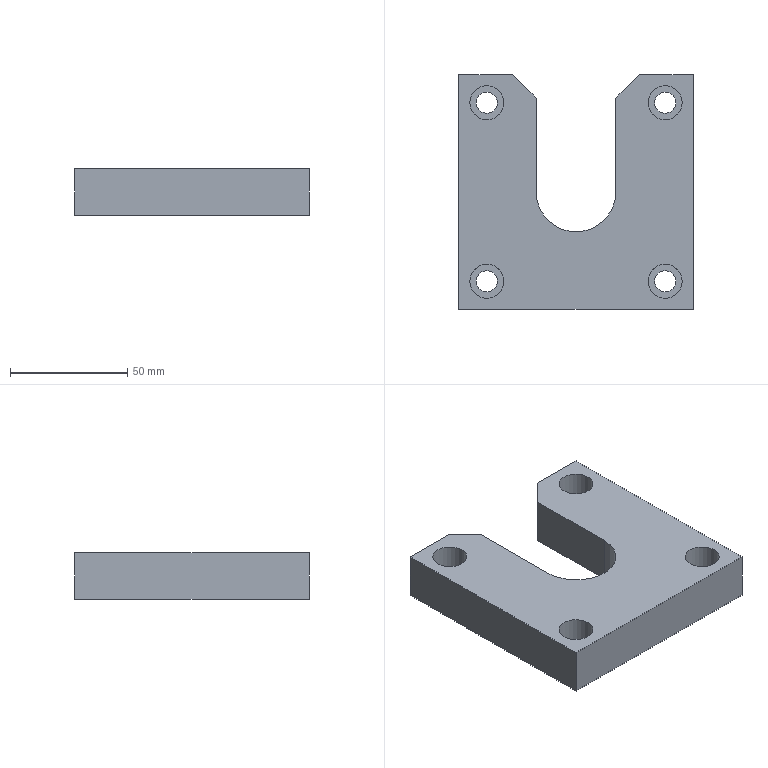Part | STEP file | lll_id890_x_t | 1 solid | 24 faces | box 100 x 100 x 20 mm | volume 145352 mm3 | plane 15 | cylinder 9 | commonest cylinder face diameters 9.009 x4 14.508 x4 34 x1
STEP:
#1=CARTESIAN_POINT('',(3772.181,632.,-360.));
#2=VERTEX_POINT('',#1);
#3=CARTESIAN_POINT('',(3779.435,632.,-360.));
#4=DIRECTION('',(0.,0.,1.));
#5=DIRECTION('',(-1.,0.,0.));
#6=AXIS2_PLACEMENT_3D('',#3,#4,#5);
#7=CIRCLE('',#6,7.254);
#8=EDGE_CURVE('',#2,#2,#7,.T.);
#9=ORIENTED_EDGE('',*,*,#8,.F.);
#10=EDGE_LOOP('',(#9));
#11=FACE_BOUND('',#10,.T.);
#12=CARTESIAN_POINT('',(3848.181,708.,-360.));
#13=VERTEX_POINT('',#12);
#14=CARTESIAN_POINT('',(3855.435,708.,-360.));
#15=DIRECTION('',(0.,0.,1.));
#16=DIRECTION('',(-1.,0.,0.));
#17=AXIS2_PLACEMENT_3D('',#14,#15,#16);
#18=CIRCLE('',#17,7.254);
#19=EDGE_CURVE('',#13,#13,#18,.T.);
#20=ORIENTED_EDGE('',*,*,#19,.F.);
#21=EDGE_LOOP('',(#20));
#22=FACE_BOUND('',#21,.T.);
#23=CARTESIAN_POINT('',(3790.435,720.,-360.));
#24=VERTEX_POINT('',#23);
#25=CARTESIAN_POINT('',(3767.435,720.,-360.));
#26=VERTEX_POINT('',#25);
#27=CARTESIAN_POINT('',(3817.435,720.,-360.));
#28=DIRECTION('',(-1.,0.,0.));
#29=VECTOR('',#28,1.);
#30=LINE('',#27,#29);
#31=EDGE_CURVE('',#24,#26,#30,.T.);
#32=ORIENTED_EDGE('',*,*,#31,.T.);
#33=CARTESIAN_POINT('',(3767.435,620.,-360.));
#34=VERTEX_POINT('',#33);
#35=CARTESIAN_POINT('',(3767.435,662.5,-360.));
#36=DIRECTION('',(0.,-1.,0.));
#37=VECTOR('',#36,1.);
#38=LINE('',#35,#37);
#39=EDGE_CURVE('',#26,#34,#38,.T.);
#40=ORIENTED_EDGE('',*,*,#39,.T.);
#41=CARTESIAN_POINT('',(3867.435,620.,-360.));
#42=VERTEX_POINT('',#41);
#43=CARTESIAN_POINT('',(3817.435,620.,-360.));
#44=DIRECTION('',(1.,0.,0.));
#45=VECTOR('',#44,1.);
#46=LINE('',#43,#45);
#47=EDGE_CURVE('',#34,#42,#46,.T.);
#48=ORIENTED_EDGE('',*,*,#47,.T.);
#49=CARTESIAN_POINT('',(3867.435,720.,-360.));
#50=VERTEX_POINT('',#49);
#51=CARTESIAN_POINT('',(3867.435,662.5,-360.));
#52=DIRECTION('',(0.,1.,0.));
#53=VECTOR('',#52,1.);
#54=LINE('',#51,#53);
#55=EDGE_CURVE('',#42,#50,#54,.T.);
#56=ORIENTED_EDGE('',*,*,#55,.T.);
#57=CARTESIAN_POINT('',(3844.435,720.,-360.));
#58=VERTEX_POINT('',#57);
#59=CARTESIAN_POINT('',(3817.435,720.,-360.));
#60=DIRECTION('',(-1.,0.,0.));
#61=VECTOR('',#60,1.);
#62=LINE('',#59,#61);
#63=EDGE_CURVE('',#50,#58,#62,.T.);
#64=ORIENTED_EDGE('',*,*,#63,.T.);
#65=CARTESIAN_POINT('',(3834.435,710.,-360.));
#66=VERTEX_POINT('',#65);
#67=CARTESIAN_POINT('',(3802.185,677.75,-360.));
#68=DIRECTION('',(-0.7071,-0.7071,0.));
#69=VECTOR('',#68,1.);
#70=LINE('',#67,#69);
#71=EDGE_CURVE('',#58,#66,#70,.T.);
#72=ORIENTED_EDGE('',*,*,#71,.T.);
#73=CARTESIAN_POINT('',(3834.435,670.,-360.));
#74=VERTEX_POINT('',#73);
#75=CARTESIAN_POINT('',(3834.435,662.5,-360.));
#76=DIRECTION('',(0.,1.,0.));
#77=VECTOR('',#76,1.);
#78=LINE('',#75,#77);
#79=EDGE_CURVE('',#74,#66,#78,.T.);
#80=ORIENTED_EDGE('',*,*,#79,.F.);
#81=CARTESIAN_POINT('',(3800.435,670.,-360.));
#82=VERTEX_POINT('',#81);
#83=CARTESIAN_POINT('',(3817.435,670.,-360.));
#84=DIRECTION('',(0.,0.,1.));
#85=DIRECTION('',(1.,0.,0.));
#86=AXIS2_PLACEMENT_3D('',#83,#84,#85);
#87=CIRCLE('',#86,17.);
#88=EDGE_CURVE('',#82,#74,#87,.T.);
#89=ORIENTED_EDGE('',*,*,#88,.F.);
#90=CARTESIAN_POINT('',(3800.435,710.,-360.));
#91=VERTEX_POINT('',#90);
#92=CARTESIAN_POINT('',(3800.435,662.5,-360.));
#93=DIRECTION('',(0.,1.,0.));
#94=VECTOR('',#93,1.);
#95=LINE('',#92,#94);
#96=EDGE_CURVE('',#82,#91,#95,.T.);
#97=ORIENTED_EDGE('',*,*,#96,.T.);
#98=CARTESIAN_POINT('',(3832.685,677.75,-360.));
#99=DIRECTION('',(0.7071,-0.7071,0.));
#100=VECTOR('',#99,1.);
#101=LINE('',#98,#100);
#102=EDGE_CURVE('',#24,#91,#101,.T.);
#103=ORIENTED_EDGE('',*,*,#102,.F.);
#104=EDGE_LOOP('',(#32,#40,#48,#56,#64,#72,#80,#89,#97,#103));
#105=FACE_BOUND('',#104,.T.);
#106=CARTESIAN_POINT('',(3848.181,632.,-360.));
#107=VERTEX_POINT('',#106);
#108=CARTESIAN_POINT('',(3855.435,632.,-360.));
#109=DIRECTION('',(0.,0.,1.));
#110=DIRECTION('',(-1.,0.,0.));
#111=AXIS2_PLACEMENT_3D('',#108,#109,#110);
#112=CIRCLE('',#111,7.254);
#113=EDGE_CURVE('',#107,#107,#112,.T.);
#114=ORIENTED_EDGE('',*,*,#113,.F.);
#115=EDGE_LOOP('',(#114));
#116=FACE_BOUND('',#115,.T.);
#117=CARTESIAN_POINT('',(3772.181,708.,-360.));
#118=VERTEX_POINT('',#117);
#119=CARTESIAN_POINT('',(3779.435,708.,-360.));
#120=DIRECTION('',(0.,0.,1.));
#121=DIRECTION('',(-1.,0.,0.));
#122=AXIS2_PLACEMENT_3D('',#119,#120,#121);
#123=CIRCLE('',#122,7.254);
#124=EDGE_CURVE('',#118,#118,#123,.T.);
#125=ORIENTED_EDGE('',*,*,#124,.F.);
#126=EDGE_LOOP('',(#125));
#127=FACE_BOUND('',#126,.T.);
#128=CARTESIAN_POINT('',(3817.435,662.5,-360.));
#129=DIRECTION('',(0.,0.,1.));
#130=DIRECTION('',(-1.,0.,0.));
#131=AXIS2_PLACEMENT_3D('',#128,#129,#130);
#132=PLANE('',#131);
#133=ADVANCED_FACE('',(#11,#22,#105,#116,#127),#132,.T.);
#134=CARTESIAN_POINT('',(3767.435,720.,-380.));
#135=VERTEX_POINT('',#134);
#136=CARTESIAN_POINT('',(3790.435,720.,-380.));
#137=VERTEX_POINT('',#136);
#138=CARTESIAN_POINT('',(3817.435,720.,-380.));
#139=DIRECTION('',(1.,0.,0.));
#140=VECTOR('',#139,1.);
#141=LINE('',#138,#140);
#142=EDGE_CURVE('',#135,#137,#141,.T.);
#143=ORIENTED_EDGE('',*,*,#142,.F.);
#144=CARTESIAN_POINT('',(3767.435,720.,-380.));
#145=DIRECTION('',(0.,0.,1.));
#146=VECTOR('',#145,1.);
#147=LINE('',#144,#146);
#148=EDGE_CURVE('',#135,#26,#147,.T.);
#149=ORIENTED_EDGE('',*,*,#148,.T.);
#150=ORIENTED_EDGE('',*,*,#31,.F.);
#151=CARTESIAN_POINT('',(3790.435,720.,-430.));
#152=DIRECTION('',(0.,0.,-1.));
#153=VECTOR('',#152,1.);
#154=LINE('',#151,#153);
#155=EDGE_CURVE('',#24,#137,#154,.T.);
#156=ORIENTED_EDGE('',*,*,#155,.T.);
#157=EDGE_LOOP('',(#143,#149,#150,#156));
#158=FACE_OUTER_BOUND('',#157,.T.);
#159=CARTESIAN_POINT('',(3817.435,720.,-380.));
#160=DIRECTION('',(0.,1.,0.));
#161=DIRECTION('',(0.,0.,1.));
#162=AXIS2_PLACEMENT_3D('',#159,#160,#161);
#163=PLANE('',#162);
#164=ADVANCED_FACE('',(#158),#163,.T.);
#165=ORIENTED_EDGE('',*,*,#63,.F.);
#166=CARTESIAN_POINT('',(3867.435,720.,-380.));
#167=VERTEX_POINT('',#166);
#168=CARTESIAN_POINT('',(3867.435,720.,-380.));
#169=DIRECTION('',(0.,0.,1.));
#170=VECTOR('',#169,1.);
#171=LINE('',#168,#170);
#172=EDGE_CURVE('',#167,#50,#171,.T.);
#173=ORIENTED_EDGE('',*,*,#172,.F.);
#174=CARTESIAN_POINT('',(3844.435,720.,-380.));
#175=VERTEX_POINT('',#174);
#176=CARTESIAN_POINT('',(3817.435,720.,-380.));
#177=DIRECTION('',(1.,0.,0.));
#178=VECTOR('',#177,1.);
#179=LINE('',#176,#178);
#180=EDGE_CURVE('',#175,#167,#179,.T.);
#181=ORIENTED_EDGE('',*,*,#180,.F.);
#182=CARTESIAN_POINT('',(3844.435,720.,-430.));
#183=DIRECTION('',(0.,0.,1.));
#184=VECTOR('',#183,1.);
#185=LINE('',#182,#184);
#186=EDGE_CURVE('',#175,#58,#185,.T.);
#187=ORIENTED_EDGE('',*,*,#186,.T.);
#188=EDGE_LOOP('',(#165,#173,#181,#187));
#189=FACE_OUTER_BOUND('',#188,.T.);
#190=CARTESIAN_POINT('',(3817.435,720.,-380.));
#191=DIRECTION('',(0.,1.,0.));
#192=DIRECTION('',(0.,0.,1.));
#193=AXIS2_PLACEMENT_3D('',#190,#191,#192);
#194=PLANE('',#193);
#195=ADVANCED_FACE('',(#189),#194,.T.);
#196=CARTESIAN_POINT('',(3774.931,708.,-380.));
#197=VERTEX_POINT('',#196);
#198=CARTESIAN_POINT('',(3779.435,708.,-380.));
#199=DIRECTION('',(0.,0.,1.));
#200=DIRECTION('',(-1.,0.,0.));
#201=AXIS2_PLACEMENT_3D('',#198,#199,#200);
#202=CIRCLE('',#201,4.505);
#203=EDGE_CURVE('',#197,#197,#202,.T.);
#204=ORIENTED_EDGE('',*,*,#203,.T.);
#205=EDGE_LOOP('',(#204));
#206=FACE_BOUND('',#205,.T.);
#207=CARTESIAN_POINT('',(3774.931,632.,-380.));
#208=VERTEX_POINT('',#207);
#209=CARTESIAN_POINT('',(3779.435,632.,-380.));
#210=DIRECTION('',(0.,0.,1.));
#211=DIRECTION('',(-1.,0.,0.));
#212=AXIS2_PLACEMENT_3D('',#209,#210,#211);
#213=CIRCLE('',#212,4.505);
#214=EDGE_CURVE('',#208,#208,#213,.T.);
#215=ORIENTED_EDGE('',*,*,#214,.T.);
#216=EDGE_LOOP('',(#215));
#217=FACE_BOUND('',#216,.T.);
#218=CARTESIAN_POINT('',(3850.931,632.,-380.));
#219=VERTEX_POINT('',#218);
#220=CARTESIAN_POINT('',(3855.435,632.,-380.));
#221=DIRECTION('',(0.,0.,1.));
#222=DIRECTION('',(-1.,0.,0.));
#223=AXIS2_PLACEMENT_3D('',#220,#221,#222);
#224=CIRCLE('',#223,4.505);
#225=EDGE_CURVE('',#219,#219,#224,.T.);
#226=ORIENTED_EDGE('',*,*,#225,.T.);
#227=EDGE_LOOP('',(#226));
#228=FACE_BOUND('',#227,.T.);
#229=CARTESIAN_POINT('',(3850.931,708.,-380.));
#230=VERTEX_POINT('',#229);
#231=CARTESIAN_POINT('',(3855.435,708.,-380.));
#232=DIRECTION('',(0.,0.,1.));
#233=DIRECTION('',(-1.,0.,0.));
#234=AXIS2_PLACEMENT_3D('',#231,#232,#233);
#235=CIRCLE('',#234,4.505);
#236=EDGE_CURVE('',#230,#230,#235,.T.);
#237=ORIENTED_EDGE('',*,*,#236,.T.);
#238=EDGE_LOOP('',(#237));
#239=FACE_BOUND('',#238,.T.);
#240=CARTESIAN_POINT('',(3800.435,670.,-380.));
#241=VERTEX_POINT('',#240);
#242=CARTESIAN_POINT('',(3800.435,710.,-380.));
#243=VERTEX_POINT('',#242);
#244=CARTESIAN_POINT('',(3800.435,662.5,-380.));
#245=DIRECTION('',(0.,1.,0.));
#246=VECTOR('',#245,1.);
#247=LINE('',#244,#246);
#248=EDGE_CURVE('',#241,#243,#247,.T.);
#249=ORIENTED_EDGE('',*,*,#248,.F.);
#250=CARTESIAN_POINT('',(3834.435,670.,-380.));
#251=VERTEX_POINT('',#250);
#252=CARTESIAN_POINT('',(3817.435,670.,-380.));
#253=DIRECTION('',(0.,0.,1.));
#254=DIRECTION('',(-1.,0.,0.));
#255=AXIS2_PLACEMENT_3D('',#252,#253,#254);
#256=CIRCLE('',#255,17.);
#257=EDGE_CURVE('',#241,#251,#256,.T.);
#258=ORIENTED_EDGE('',*,*,#257,.T.);
#259=CARTESIAN_POINT('',(3834.435,710.,-380.));
#260=VERTEX_POINT('',#259);
#261=CARTESIAN_POINT('',(3834.435,662.5,-380.));
#262=DIRECTION('',(0.,1.,0.));
#263=VECTOR('',#262,1.);
#264=LINE('',#261,#263);
#265=EDGE_CURVE('',#251,#260,#264,.T.);
#266=ORIENTED_EDGE('',*,*,#265,.T.);
#267=CARTESIAN_POINT('',(3802.185,677.75,-380.));
#268=DIRECTION('',(0.7071,0.7071,0.));
#269=VECTOR('',#268,1.);
#270=LINE('',#267,#269);
#271=EDGE_CURVE('',#260,#175,#270,.T.);
#272=ORIENTED_EDGE('',*,*,#271,.T.);
#273=ORIENTED_EDGE('',*,*,#180,.T.);
#274=CARTESIAN_POINT('',(3867.435,620.,-380.));
#275=VERTEX_POINT('',#274);
#276=CARTESIAN_POINT('',(3867.435,662.5,-380.));
#277=DIRECTION('',(0.,-1.,0.));
#278=VECTOR('',#277,1.);
#279=LINE('',#276,#278);
#280=EDGE_CURVE('',#167,#275,#279,.T.);
#281=ORIENTED_EDGE('',*,*,#280,.T.);
#282=CARTESIAN_POINT('',(3767.435,620.,-380.));
#283=VERTEX_POINT('',#282);
#284=CARTESIAN_POINT('',(3817.435,620.,-380.));
#285=DIRECTION('',(-1.,0.,0.));
#286=VECTOR('',#285,1.);
#287=LINE('',#284,#286);
#288=EDGE_CURVE('',#275,#283,#287,.T.);
#289=ORIENTED_EDGE('',*,*,#288,.T.);
#290=CARTESIAN_POINT('',(3767.435,662.5,-380.));
#291=DIRECTION('',(0.,1.,0.));
#292=VECTOR('',#291,1.);
#293=LINE('',#290,#292);
#294=EDGE_CURVE('',#283,#135,#293,.T.);
#295=ORIENTED_EDGE('',*,*,#294,.T.);
#296=ORIENTED_EDGE('',*,*,#142,.T.);
#297=CARTESIAN_POINT('',(3832.685,677.75,-380.));
#298=DIRECTION('',(-0.7071,0.7071,0.));
#299=VECTOR('',#298,1.);
#300=LINE('',#297,#299);
#301=EDGE_CURVE('',#243,#137,#300,.T.);
#302=ORIENTED_EDGE('',*,*,#301,.F.);
#303=EDGE_LOOP('',(#249,#258,#266,#272,#273,#281,#289,#295,#296,#302));
#304=FACE_BOUND('',#303,.T.);
#305=CARTESIAN_POINT('',(3817.435,662.5,-380.));
#306=DIRECTION('',(0.,0.,-1.));
#307=DIRECTION('',(1.,0.,0.));
#308=AXIS2_PLACEMENT_3D('',#305,#306,#307);
#309=PLANE('',#308);
#310=ADVANCED_FACE('',(#206,#217,#228,#239,#304),#309,.T.);
#311=ORIENTED_EDGE('',*,*,#148,.F.);
#312=ORIENTED_EDGE('',*,*,#294,.F.);
#313=CARTESIAN_POINT('',(3767.435,620.,-380.));
#314=DIRECTION('',(0.,0.,1.));
#315=VECTOR('',#314,1.);
#316=LINE('',#313,#315);
#317=EDGE_CURVE('',#283,#34,#316,.T.);
#318=ORIENTED_EDGE('',*,*,#317,.T.);
#319=ORIENTED_EDGE('',*,*,#39,.F.);
#320=EDGE_LOOP('',(#311,#312,#318,#319));
#321=FACE_OUTER_BOUND('',#320,.T.);
#322=CARTESIAN_POINT('',(3767.435,662.5,-380.));
#323=DIRECTION('',(-1.,0.,0.));
#324=DIRECTION('',(0.,0.,-1.));
#325=AXIS2_PLACEMENT_3D('',#322,#323,#324);
#326=PLANE('',#325);
#327=ADVANCED_FACE('',(#321),#326,.T.);
#328=ORIENTED_EDGE('',*,*,#317,.F.);
#329=ORIENTED_EDGE('',*,*,#288,.F.);
#330=CARTESIAN_POINT('',(3867.435,620.,-380.));
#331=DIRECTION('',(0.,0.,1.));
#332=VECTOR('',#331,1.);
#333=LINE('',#330,#332);
#334=EDGE_CURVE('',#275,#42,#333,.T.);
#335=ORIENTED_EDGE('',*,*,#334,.T.);
#336=ORIENTED_EDGE('',*,*,#47,.F.);
#337=EDGE_LOOP('',(#328,#329,#335,#336));
#338=FACE_OUTER_BOUND('',#337,.T.);
#339=CARTESIAN_POINT('',(3817.435,620.,-380.));
#340=DIRECTION('',(0.,-1.,0.));
#341=DIRECTION('',(0.,0.,-1.));
#342=AXIS2_PLACEMENT_3D('',#339,#340,#341);
#343=PLANE('',#342);
#344=ADVANCED_FACE('',(#338),#343,.T.);
#345=ORIENTED_EDGE('',*,*,#280,.F.);
#346=ORIENTED_EDGE('',*,*,#172,.T.);
#347=ORIENTED_EDGE('',*,*,#55,.F.);
#348=ORIENTED_EDGE('',*,*,#334,.F.);
#349=EDGE_LOOP('',(#345,#346,#347,#348));
#350=FACE_OUTER_BOUND('',#349,.T.);
#351=CARTESIAN_POINT('',(3867.435,662.5,-380.));
#352=DIRECTION('',(1.,0.,0.));
#353=DIRECTION('',(0.,0.,1.));
#354=AXIS2_PLACEMENT_3D('',#351,#352,#353);
#355=PLANE('',#354);
#356=ADVANCED_FACE('',(#350),#355,.T.);
#357=ORIENTED_EDGE('',*,*,#102,.T.);
#358=CARTESIAN_POINT('',(3800.435,710.,-430.));
#359=DIRECTION('',(0.,0.,1.));
#360=VECTOR('',#359,1.);
#361=LINE('',#358,#360);
#362=EDGE_CURVE('',#243,#91,#361,.T.);
#363=ORIENTED_EDGE('',*,*,#362,.F.);
#364=ORIENTED_EDGE('',*,*,#301,.T.);
#365=ORIENTED_EDGE('',*,*,#155,.F.);
#366=EDGE_LOOP('',(#357,#363,#364,#365));
#367=FACE_OUTER_BOUND('',#366,.T.);
#368=CARTESIAN_POINT('',(3790.435,720.,-430.));
#369=DIRECTION('',(0.7071,0.7071,0.));
#370=DIRECTION('',(-0.7071,0.7071,0.));
#371=AXIS2_PLACEMENT_3D('',#368,#369,#370);
#372=PLANE('',#371);
#373=ADVANCED_FACE('',(#367),#372,.T.);
#374=ORIENTED_EDGE('',*,*,#96,.F.);
#375=CARTESIAN_POINT('',(3800.435,670.,-430.));
#376=DIRECTION('',(0.,0.,1.));
#377=VECTOR('',#376,1.);
#378=LINE('',#375,#377);
#379=EDGE_CURVE('',#241,#82,#378,.T.);
#380=ORIENTED_EDGE('',*,*,#379,.F.);
#381=ORIENTED_EDGE('',*,*,#248,.T.);
#382=ORIENTED_EDGE('',*,*,#362,.T.);
#383=EDGE_LOOP('',(#374,#380,#381,#382));
#384=FACE_OUTER_BOUND('',#383,.T.);
#385=CARTESIAN_POINT('',(3800.435,710.,-430.));
#386=DIRECTION('',(1.,0.,0.));
#387=DIRECTION('',(0.,1.,0.));
#388=AXIS2_PLACEMENT_3D('',#385,#386,#387);
#389=PLANE('',#388);
#390=ADVANCED_FACE('',(#384),#389,.T.);
#391=ORIENTED_EDGE('',*,*,#88,.T.);
#392=CARTESIAN_POINT('',(3834.435,670.,-430.));
#393=DIRECTION('',(0.,0.,1.));
#394=VECTOR('',#393,1.);
#395=LINE('',#392,#394);
#396=EDGE_CURVE('',#251,#74,#395,.T.);
#397=ORIENTED_EDGE('',*,*,#396,.F.);
#398=ORIENTED_EDGE('',*,*,#257,.F.);
#399=ORIENTED_EDGE('',*,*,#379,.T.);
#400=EDGE_LOOP('',(#391,#397,#398,#399));
#401=FACE_OUTER_BOUND('',#400,.T.);
#402=CARTESIAN_POINT('',(3817.435,670.,-430.));
#403=DIRECTION('',(0.,0.,1.));
#404=DIRECTION('',(-1.,0.,0.));
#405=AXIS2_PLACEMENT_3D('',#402,#403,#404);
#406=CYLINDRICAL_SURFACE('',#405,17.);
#407=ADVANCED_FACE('',(#401),#406,.F.);
#408=ORIENTED_EDGE('',*,*,#79,.T.);
#409=CARTESIAN_POINT('',(3834.435,710.,-430.));
#410=DIRECTION('',(0.,0.,1.));
#411=VECTOR('',#410,1.);
#412=LINE('',#409,#411);
#413=EDGE_CURVE('',#260,#66,#412,.T.);
#414=ORIENTED_EDGE('',*,*,#413,.F.);
#415=ORIENTED_EDGE('',*,*,#265,.F.);
#416=ORIENTED_EDGE('',*,*,#396,.T.);
#417=EDGE_LOOP('',(#408,#414,#415,#416));
#418=FACE_OUTER_BOUND('',#417,.T.);
#419=CARTESIAN_POINT('',(3834.435,670.,-430.));
#420=DIRECTION('',(-1.,0.,0.));
#421=DIRECTION('',(0.,-1.,0.));
#422=AXIS2_PLACEMENT_3D('',#419,#420,#421);
#423=PLANE('',#422);
#424=ADVANCED_FACE('',(#418),#423,.T.);
#425=ORIENTED_EDGE('',*,*,#71,.F.);
#426=ORIENTED_EDGE('',*,*,#186,.F.);
#427=ORIENTED_EDGE('',*,*,#271,.F.);
#428=ORIENTED_EDGE('',*,*,#413,.T.);
#429=EDGE_LOOP('',(#425,#426,#427,#428));
#430=FACE_OUTER_BOUND('',#429,.T.);
#431=CARTESIAN_POINT('',(3834.435,710.,-430.));
#432=DIRECTION('',(-0.7071,0.7071,0.));
#433=DIRECTION('',(-0.7071,-0.7071,0.));
#434=AXIS2_PLACEMENT_3D('',#431,#432,#433);
#435=PLANE('',#434);
#436=ADVANCED_FACE('',(#430),#435,.T.);
#437=ORIENTED_EDGE('',*,*,#236,.F.);
#438=EDGE_LOOP('',(#437));
#439=FACE_BOUND('',#438,.T.);
#440=CARTESIAN_POINT('',(3850.931,708.,-371.));
#441=VERTEX_POINT('',#440);
#442=CARTESIAN_POINT('',(3855.435,708.,-371.));
#443=DIRECTION('',(0.,0.,1.));
#444=DIRECTION('',(-1.,0.,0.));
#445=AXIS2_PLACEMENT_3D('',#442,#443,#444);
#446=CIRCLE('',#445,4.505);
#447=EDGE_CURVE('',#441,#441,#446,.T.);
#448=ORIENTED_EDGE('',*,*,#447,.T.);
#449=EDGE_LOOP('',(#448));
#450=FACE_BOUND('',#449,.T.);
#451=CARTESIAN_POINT('',(3855.435,708.,-358.));
#452=DIRECTION('',(0.,0.,-1.));
#453=DIRECTION('',(1.,0.,0.));
#454=AXIS2_PLACEMENT_3D('',#451,#452,#453);
#455=CYLINDRICAL_SURFACE('',#454,4.505);
#456=ADVANCED_FACE('',(#439,#450),#455,.F.);
#457=ORIENTED_EDGE('',*,*,#447,.F.);
#458=EDGE_LOOP('',(#457));
#459=FACE_BOUND('',#458,.T.);
#460=CARTESIAN_POINT('',(3848.181,708.,-371.));
#461=VERTEX_POINT('',#460);
#462=CARTESIAN_POINT('',(3855.435,708.,-371.));
#463=DIRECTION('',(0.,0.,1.));
#464=DIRECTION('',(-1.,0.,0.));
#465=AXIS2_PLACEMENT_3D('',#462,#463,#464);
#466=CIRCLE('',#465,7.254);
#467=EDGE_CURVE('',#461,#461,#466,.T.);
#468=ORIENTED_EDGE('',*,*,#467,.T.);
#469=EDGE_LOOP('',(#468));
#470=FACE_BOUND('',#469,.T.);
#471=CARTESIAN_POINT('',(3855.435,708.,-371.));
#472=DIRECTION('',(0.,0.,-1.));
#473=DIRECTION('',(1.,0.,0.));
#474=AXIS2_PLACEMENT_3D('',#471,#472,#473);
#475=PLANE('',#474);
#476=ADVANCED_FACE('',(#459,#470),#475,.F.);
#477=ORIENTED_EDGE('',*,*,#467,.F.);
#478=EDGE_LOOP('',(#477));
#479=FACE_BOUND('',#478,.T.);
#480=ORIENTED_EDGE('',*,*,#19,.T.);
#481=EDGE_LOOP('',(#480));
#482=FACE_BOUND('',#481,.T.);
#483=CARTESIAN_POINT('',(3855.435,708.,-360.));
#484=DIRECTION('',(0.,0.,-1.));
#485=DIRECTION('',(1.,0.,0.));
#486=AXIS2_PLACEMENT_3D('',#483,#484,#485);
#487=CYLINDRICAL_SURFACE('',#486,7.254);
#488=ADVANCED_FACE('',(#479,#482),#487,.F.);
#489=ORIENTED_EDGE('',*,*,#225,.F.);
#490=EDGE_LOOP('',(#489));
#491=FACE_BOUND('',#490,.T.);
#492=CARTESIAN_POINT('',(3850.931,632.,-371.));
#493=VERTEX_POINT('',#492);
#494=CARTESIAN_POINT('',(3855.435,632.,-371.));
#495=DIRECTION('',(0.,0.,1.));
#496=DIRECTION('',(-1.,0.,0.));
#497=AXIS2_PLACEMENT_3D('',#494,#495,#496);
#498=CIRCLE('',#497,4.505);
#499=EDGE_CURVE('',#493,#493,#498,.T.);
#500=ORIENTED_EDGE('',*,*,#499,.T.);
#501=EDGE_LOOP('',(#500));
#502=FACE_BOUND('',#501,.T.);
#503=CARTESIAN_POINT('',(3855.435,632.,-358.));
#504=DIRECTION('',(0.,0.,-1.));
#505=DIRECTION('',(1.,0.,0.));
#506=AXIS2_PLACEMENT_3D('',#503,#504,#505);
#507=CYLINDRICAL_SURFACE('',#506,4.505);
#508=ADVANCED_FACE('',(#491,#502),#507,.F.);
#509=ORIENTED_EDGE('',*,*,#499,.F.);
#510=EDGE_LOOP('',(#509));
#511=FACE_BOUND('',#510,.T.);
#512=CARTESIAN_POINT('',(3848.181,632.,-371.));
#513=VERTEX_POINT('',#512);
#514=CARTESIAN_POINT('',(3855.435,632.,-371.));
#515=DIRECTION('',(0.,0.,1.));
#516=DIRECTION('',(-1.,0.,0.));
#517=AXIS2_PLACEMENT_3D('',#514,#515,#516);
#518=CIRCLE('',#517,7.254);
#519=EDGE_CURVE('',#513,#513,#518,.T.);
#520=ORIENTED_EDGE('',*,*,#519,.T.);
#521=EDGE_LOOP('',(#520));
#522=FACE_BOUND('',#521,.T.);
#523=CARTESIAN_POINT('',(3855.435,632.,-371.));
#524=DIRECTION('',(0.,0.,-1.));
#525=DIRECTION('',(1.,0.,0.));
#526=AXIS2_PLACEMENT_3D('',#523,#524,#525);
#527=PLANE('',#526);
#528=ADVANCED_FACE('',(#511,#522),#527,.F.);
#529=ORIENTED_EDGE('',*,*,#519,.F.);
#530=EDGE_LOOP('',(#529));
#531=FACE_BOUND('',#530,.T.);
#532=ORIENTED_EDGE('',*,*,#113,.T.);
#533=EDGE_LOOP('',(#532));
#534=FACE_BOUND('',#533,.T.);
#535=CARTESIAN_POINT('',(3855.435,632.,-360.));
#536=DIRECTION('',(0.,0.,-1.));
#537=DIRECTION('',(1.,0.,0.));
#538=AXIS2_PLACEMENT_3D('',#535,#536,#537);
#539=CYLINDRICAL_SURFACE('',#538,7.254);
#540=ADVANCED_FACE('',(#531,#534),#539,.F.);
#541=ORIENTED_EDGE('',*,*,#214,.F.);
#542=EDGE_LOOP('',(#541));
#543=FACE_BOUND('',#542,.T.);
#544=CARTESIAN_POINT('',(3774.931,632.,-371.));
#545=VERTEX_POINT('',#544);
#546=CARTESIAN_POINT('',(3779.435,632.,-371.));
#547=DIRECTION('',(0.,0.,1.));
#548=DIRECTION('',(-1.,0.,0.));
#549=AXIS2_PLACEMENT_3D('',#546,#547,#548);
#550=CIRCLE('',#549,4.505);
#551=EDGE_CURVE('',#545,#545,#550,.T.);
#552=ORIENTED_EDGE('',*,*,#551,.T.);
#553=EDGE_LOOP('',(#552));
#554=FACE_BOUND('',#553,.T.);
#555=CARTESIAN_POINT('',(3779.435,632.,-358.));
#556=DIRECTION('',(0.,0.,-1.));
#557=DIRECTION('',(1.,0.,0.));
#558=AXIS2_PLACEMENT_3D('',#555,#556,#557);
#559=CYLINDRICAL_SURFACE('',#558,4.505);
#560=ADVANCED_FACE('',(#543,#554),#559,.F.);
#561=ORIENTED_EDGE('',*,*,#551,.F.);
#562=EDGE_LOOP('',(#561));
#563=FACE_BOUND('',#562,.T.);
#564=CARTESIAN_POINT('',(3772.181,632.,-371.));
#565=VERTEX_POINT('',#564);
#566=CARTESIAN_POINT('',(3779.435,632.,-371.));
#567=DIRECTION('',(0.,0.,1.));
#568=DIRECTION('',(-1.,0.,0.));
#569=AXIS2_PLACEMENT_3D('',#566,#567,#568);
#570=CIRCLE('',#569,7.254);
#571=EDGE_CURVE('',#565,#565,#570,.T.);
#572=ORIENTED_EDGE('',*,*,#571,.T.);
#573=EDGE_LOOP('',(#572));
#574=FACE_BOUND('',#573,.T.);
#575=CARTESIAN_POINT('',(3779.435,632.,-371.));
#576=DIRECTION('',(0.,0.,-1.));
#577=DIRECTION('',(1.,0.,0.));
#578=AXIS2_PLACEMENT_3D('',#575,#576,#577);
#579=PLANE('',#578);
#580=ADVANCED_FACE('',(#563,#574),#579,.F.);
#581=ORIENTED_EDGE('',*,*,#571,.F.);
#582=EDGE_LOOP('',(#581));
#583=FACE_BOUND('',#582,.T.);
#584=ORIENTED_EDGE('',*,*,#8,.T.);
#585=EDGE_LOOP('',(#584));
#586=FACE_BOUND('',#585,.T.);
#587=CARTESIAN_POINT('',(3779.435,632.,-360.));
#588=DIRECTION('',(0.,0.,-1.));
#589=DIRECTION('',(1.,0.,0.));
#590=AXIS2_PLACEMENT_3D('',#587,#588,#589);
#591=CYLINDRICAL_SURFACE('',#590,7.254);
#592=ADVANCED_FACE('',(#583,#586),#591,.F.);
#593=ORIENTED_EDGE('',*,*,#203,.F.);
#594=EDGE_LOOP('',(#593));
#595=FACE_BOUND('',#594,.T.);
#596=CARTESIAN_POINT('',(3774.931,708.,-371.));
#597=VERTEX_POINT('',#596);
#598=CARTESIAN_POINT('',(3779.435,708.,-371.));
#599=DIRECTION('',(0.,0.,1.));
#600=DIRECTION('',(-1.,0.,0.));
#601=AXIS2_PLACEMENT_3D('',#598,#599,#600);
#602=CIRCLE('',#601,4.505);
#603=EDGE_CURVE('',#597,#597,#602,.T.);
#604=ORIENTED_EDGE('',*,*,#603,.T.);
#605=EDGE_LOOP('',(#604));
#606=FACE_BOUND('',#605,.T.);
#607=CARTESIAN_POINT('',(3779.435,708.,-358.));
#608=DIRECTION('',(0.,0.,-1.));
#609=DIRECTION('',(1.,0.,0.));
#610=AXIS2_PLACEMENT_3D('',#607,#608,#609);
#611=CYLINDRICAL_SURFACE('',#610,4.505);
#612=ADVANCED_FACE('',(#595,#606),#611,.F.);
#613=ORIENTED_EDGE('',*,*,#603,.F.);
#614=EDGE_LOOP('',(#613));
#615=FACE_BOUND('',#614,.T.);
#616=CARTESIAN_POINT('',(3772.181,708.,-371.));
#617=VERTEX_POINT('',#616);
#618=CARTESIAN_POINT('',(3779.435,708.,-371.));
#619=DIRECTION('',(0.,0.,1.));
#620=DIRECTION('',(-1.,0.,0.));
#621=AXIS2_PLACEMENT_3D('',#618,#619,#620);
#622=CIRCLE('',#621,7.254);
#623=EDGE_CURVE('',#617,#617,#622,.T.);
#624=ORIENTED_EDGE('',*,*,#623,.T.);
#625=EDGE_LOOP('',(#624));
#626=FACE_BOUND('',#625,.T.);
#627=CARTESIAN_POINT('',(3779.435,708.,-371.));
#628=DIRECTION('',(0.,0.,-1.));
#629=DIRECTION('',(1.,0.,0.));
#630=AXIS2_PLACEMENT_3D('',#627,#628,#629);
#631=PLANE('',#630);
#632=ADVANCED_FACE('',(#615,#626),#631,.F.);
#633=ORIENTED_EDGE('',*,*,#623,.F.);
#634=EDGE_LOOP('',(#633));
#635=FACE_BOUND('',#634,.T.);
#636=ORIENTED_EDGE('',*,*,#124,.T.);
#637=EDGE_LOOP('',(#636));
#638=FACE_BOUND('',#637,.T.);
#639=CARTESIAN_POINT('',(3779.435,708.,-360.));
#640=DIRECTION('',(0.,0.,-1.));
#641=DIRECTION('',(1.,0.,0.));
#642=AXIS2_PLACEMENT_3D('',#639,#640,#641);
#643=CYLINDRICAL_SURFACE('',#642,7.254);
#644=ADVANCED_FACE('',(#635,#638),#643,.F.);
#645=CLOSED_SHELL('',(#133,#164,#195,#310,#327,#344,#356,#373,#390,#407,#424,#436,#456,#476,#488,#508,#528,#540,#560,#580,#592,#612,#632,#644));
#646=MANIFOLD_SOLID_BREP('',#645);
#647=(LENGTH_UNIT()NAMED_UNIT(*)SI_UNIT(.MILLI.,.METRE.));
#648=UNCERTAINTY_MEASURE_WITH_UNIT(LENGTH_MEASURE(0.00002),#647,'','');
#649=(NAMED_UNIT(*)PLANE_ANGLE_UNIT()SI_UNIT($,.RADIAN.));
#650=PLANE_ANGLE_MEASURE_WITH_UNIT(PLANE_ANGLE_MEASURE(0.01745),#649);
#651=DIMENSIONAL_EXPONENTS(0.,0.,0.,0.,0.,0.,0.);
#652=(CONVERSION_BASED_UNIT('DEGREE',#650)NAMED_UNIT(#651)PLANE_ANGLE_UNIT());
#653=(NAMED_UNIT(*)SI_UNIT($,.STERADIAN.)SOLID_ANGLE_UNIT());
#654=(GEOMETRIC_REPRESENTATION_CONTEXT(3)GLOBAL_UNCERTAINTY_ASSIGNED_CONTEXT((#648))GLOBAL_UNIT_ASSIGNED_CONTEXT((#647,#652,#653))REPRESENTATION_CONTEXT('',''));
#655=ADVANCED_BREP_SHAPE_REPRESENTATION('',(#646),#654);